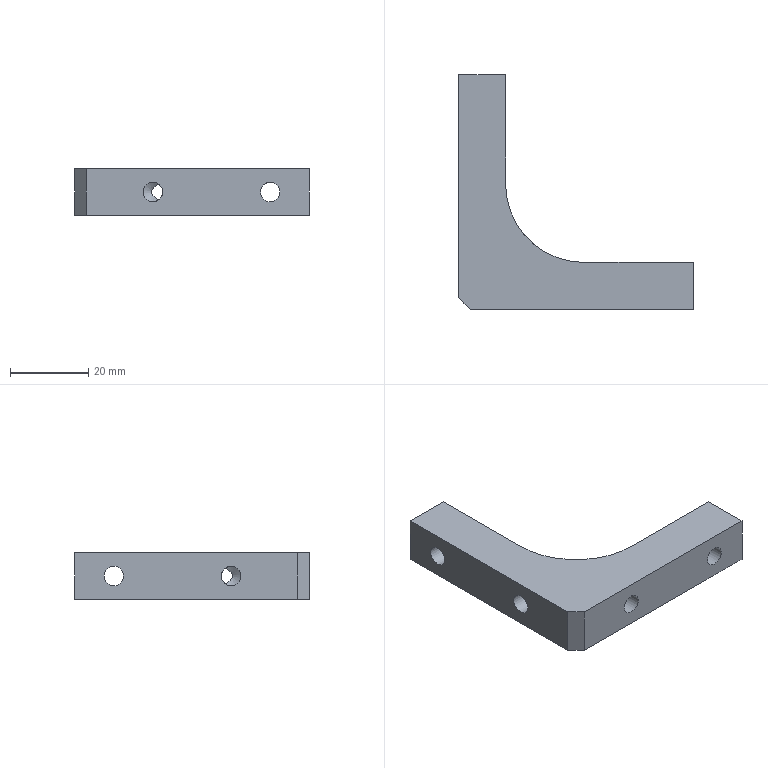Part | NX | 1 solid | 16 faces | box 60 x 60 x 12 mm | volume 15454 mm3 | plane 9 | cylinder 5 | cone 2 | commonest cylinder face diameters 5 x4 40 x1
STEP:
#1=CARTESIAN_POINT('',(12.,60.,-6.));
#2=VERTEX_POINT('',#1);
#3=CARTESIAN_POINT('',(0.,60.,-6.));
#4=VERTEX_POINT('',#3);
#5=CARTESIAN_POINT('',(12.,60.,-6.));
#6=DIRECTION('',(-1.,0.,0.));
#7=VECTOR('',#6,1000.);
#8=LINE('',#5,#7);
#9=EDGE_CURVE('',#2,#4,#8,.T.);
#10=ORIENTED_EDGE('',*,*,#9,.T.);
#11=CARTESIAN_POINT('',(0.,60.,6.));
#12=VERTEX_POINT('',#11);
#13=CARTESIAN_POINT('',(0.,60.,6.));
#14=DIRECTION('',(0.,0.,-1.));
#15=VECTOR('',#14,1000.);
#16=LINE('',#13,#15);
#17=EDGE_CURVE('',#12,#4,#16,.T.);
#18=ORIENTED_EDGE('',*,*,#17,.F.);
#19=CARTESIAN_POINT('',(12.,60.,6.));
#20=VERTEX_POINT('',#19);
#21=CARTESIAN_POINT('',(12.,60.,6.));
#22=DIRECTION('',(-1.,0.,0.));
#23=VECTOR('',#22,1000.);
#24=LINE('',#21,#23);
#25=EDGE_CURVE('',#20,#12,#24,.T.);
#26=ORIENTED_EDGE('',*,*,#25,.F.);
#27=CARTESIAN_POINT('',(12.,60.,6.));
#28=DIRECTION('',(0.,0.,-1.));
#29=VECTOR('',#28,1000.);
#30=LINE('',#27,#29);
#31=EDGE_CURVE('',#20,#2,#30,.T.);
#32=ORIENTED_EDGE('',*,*,#31,.T.);
#33=EDGE_LOOP('',(#10,#18,#26,#32));
#34=FACE_BOUND('',#33,.T.);
#35=CARTESIAN_POINT('',(12.,60.,6.));
#36=DIRECTION('',(0.,-1.,0.));
#37=DIRECTION('',(1.,0.,0.));
#38=AXIS2_PLACEMENT_3D('',#35,#36,#37);
#39=PLANE('',#38);
#40=ADVANCED_FACE('',(#34),#39,.F.);
#41=CARTESIAN_POINT('',(0.,20.,2.5));
#42=VERTEX_POINT('',#41);
#43=CARTESIAN_POINT('',(0.,20.,0.));
#44=DIRECTION('',(-1.,0.,0.));
#45=DIRECTION('',(0.,0.,1.));
#46=AXIS2_PLACEMENT_3D('',#43,#44,#45);
#47=CIRCLE('',#46,2.5);
#48=EDGE_CURVE('',#42,#42,#47,.T.);
#49=ORIENTED_EDGE('',*,*,#48,.F.);
#50=EDGE_LOOP('',(#49));
#51=FACE_BOUND('',#50,.T.);
#52=CARTESIAN_POINT('',(0.,50.,2.5));
#53=VERTEX_POINT('',#52);
#54=CARTESIAN_POINT('',(0.,50.,0.));
#55=DIRECTION('',(-1.,0.,0.));
#56=DIRECTION('',(0.,0.,1.));
#57=AXIS2_PLACEMENT_3D('',#54,#55,#56);
#58=CIRCLE('',#57,2.5);
#59=EDGE_CURVE('',#53,#53,#58,.T.);
#60=ORIENTED_EDGE('',*,*,#59,.F.);
#61=EDGE_LOOP('',(#60));
#62=FACE_BOUND('',#61,.T.);
#63=CARTESIAN_POINT('',(0.,3.,-6.));
#64=VERTEX_POINT('',#63);
#65=CARTESIAN_POINT('',(0.,60.,-6.));
#66=DIRECTION('',(0.,-1.,0.));
#67=VECTOR('',#66,1000.);
#68=LINE('',#65,#67);
#69=EDGE_CURVE('',#4,#64,#68,.T.);
#70=ORIENTED_EDGE('',*,*,#69,.T.);
#71=CARTESIAN_POINT('',(0.,3.,6.));
#72=VERTEX_POINT('',#71);
#73=CARTESIAN_POINT('',(0.,3.,6.));
#74=DIRECTION('',(0.,0.,1.));
#75=VECTOR('',#74,1000.);
#76=LINE('',#73,#75);
#77=EDGE_CURVE('',#64,#72,#76,.T.);
#78=ORIENTED_EDGE('',*,*,#77,.T.);
#79=CARTESIAN_POINT('',(0.,60.,6.));
#80=DIRECTION('',(0.,-1.,0.));
#81=VECTOR('',#80,1000.);
#82=LINE('',#79,#81);
#83=EDGE_CURVE('',#12,#72,#82,.T.);
#84=ORIENTED_EDGE('',*,*,#83,.F.);
#85=ORIENTED_EDGE('',*,*,#17,.T.);
#86=EDGE_LOOP('',(#70,#78,#84,#85));
#87=FACE_BOUND('',#86,.T.);
#88=CARTESIAN_POINT('',(0.,60.,6.));
#89=DIRECTION('',(1.,0.,0.));
#90=DIRECTION('',(0.,1.,0.));
#91=AXIS2_PLACEMENT_3D('',#88,#89,#90);
#92=PLANE('',#91);
#93=ADVANCED_FACE('',(#51,#62,#87),#92,.F.);
#94=CARTESIAN_POINT('',(20.,0.,-2.5));
#95=VERTEX_POINT('',#94);
#96=CARTESIAN_POINT('',(20.,0.,0.));
#97=DIRECTION('',(0.,-1.,0.));
#98=DIRECTION('',(0.,0.,-1.));
#99=AXIS2_PLACEMENT_3D('',#96,#97,#98);
#100=CIRCLE('',#99,2.5);
#101=EDGE_CURVE('',#95,#95,#100,.T.);
#102=ORIENTED_EDGE('',*,*,#101,.F.);
#103=EDGE_LOOP('',(#102));
#104=FACE_BOUND('',#103,.T.);
#105=CARTESIAN_POINT('',(50.,0.,-2.5));
#106=VERTEX_POINT('',#105);
#107=CARTESIAN_POINT('',(50.,0.,0.));
#108=DIRECTION('',(0.,-1.,0.));
#109=DIRECTION('',(0.,0.,-1.));
#110=AXIS2_PLACEMENT_3D('',#107,#108,#109);
#111=CIRCLE('',#110,2.5);
#112=EDGE_CURVE('',#106,#106,#111,.T.);
#113=ORIENTED_EDGE('',*,*,#112,.F.);
#114=EDGE_LOOP('',(#113));
#115=FACE_BOUND('',#114,.T.);
#116=CARTESIAN_POINT('',(3.,0.,6.));
#117=VERTEX_POINT('',#116);
#118=CARTESIAN_POINT('',(60.,0.,6.));
#119=VERTEX_POINT('',#118);
#120=CARTESIAN_POINT('',(0.,0.,6.));
#121=DIRECTION('',(1.,0.,0.));
#122=VECTOR('',#121,1000.);
#123=LINE('',#120,#122);
#124=EDGE_CURVE('',#117,#119,#123,.T.);
#125=ORIENTED_EDGE('',*,*,#124,.F.);
#126=CARTESIAN_POINT('',(3.,0.,-6.));
#127=VERTEX_POINT('',#126);
#128=CARTESIAN_POINT('',(3.,0.,6.));
#129=DIRECTION('',(0.,0.,-1.));
#130=VECTOR('',#129,1000.);
#131=LINE('',#128,#130);
#132=EDGE_CURVE('',#117,#127,#131,.T.);
#133=ORIENTED_EDGE('',*,*,#132,.T.);
#134=CARTESIAN_POINT('',(60.,0.,-6.));
#135=VERTEX_POINT('',#134);
#136=CARTESIAN_POINT('',(0.,0.,-6.));
#137=DIRECTION('',(1.,0.,0.));
#138=VECTOR('',#137,1000.);
#139=LINE('',#136,#138);
#140=EDGE_CURVE('',#127,#135,#139,.T.);
#141=ORIENTED_EDGE('',*,*,#140,.T.);
#142=CARTESIAN_POINT('',(60.,0.,6.));
#143=DIRECTION('',(0.,0.,-1.));
#144=VECTOR('',#143,1000.);
#145=LINE('',#142,#144);
#146=EDGE_CURVE('',#119,#135,#145,.T.);
#147=ORIENTED_EDGE('',*,*,#146,.F.);
#148=EDGE_LOOP('',(#125,#133,#141,#147));
#149=FACE_BOUND('',#148,.T.);
#150=CARTESIAN_POINT('',(0.,0.,6.));
#151=DIRECTION('',(0.,1.,0.));
#152=DIRECTION('',(-1.,0.,0.));
#153=AXIS2_PLACEMENT_3D('',#150,#151,#152);
#154=PLANE('',#153);
#155=ADVANCED_FACE('',(#104,#115,#149),#154,.F.);
#156=CARTESIAN_POINT('',(60.,12.,-6.));
#157=VERTEX_POINT('',#156);
#158=CARTESIAN_POINT('',(60.,0.,-6.));
#159=DIRECTION('',(0.,1.,0.));
#160=VECTOR('',#159,1000.);
#161=LINE('',#158,#160);
#162=EDGE_CURVE('',#135,#157,#161,.T.);
#163=ORIENTED_EDGE('',*,*,#162,.T.);
#164=CARTESIAN_POINT('',(60.,12.,6.));
#165=VERTEX_POINT('',#164);
#166=CARTESIAN_POINT('',(60.,12.,6.));
#167=DIRECTION('',(0.,0.,-1.));
#168=VECTOR('',#167,1000.);
#169=LINE('',#166,#168);
#170=EDGE_CURVE('',#165,#157,#169,.T.);
#171=ORIENTED_EDGE('',*,*,#170,.F.);
#172=CARTESIAN_POINT('',(60.,0.,6.));
#173=DIRECTION('',(0.,1.,0.));
#174=VECTOR('',#173,1000.);
#175=LINE('',#172,#174);
#176=EDGE_CURVE('',#119,#165,#175,.T.);
#177=ORIENTED_EDGE('',*,*,#176,.F.);
#178=ORIENTED_EDGE('',*,*,#146,.T.);
#179=EDGE_LOOP('',(#163,#171,#177,#178));
#180=FACE_BOUND('',#179,.T.);
#181=CARTESIAN_POINT('',(60.,0.,6.));
#182=DIRECTION('',(-1.,0.,0.));
#183=DIRECTION('',(0.,-1.,0.));
#184=AXIS2_PLACEMENT_3D('',#181,#182,#183);
#185=PLANE('',#184);
#186=ADVANCED_FACE('',(#180),#185,.F.);
#187=CARTESIAN_POINT('',(52.5,12.,0.));
#188=VERTEX_POINT('',#187);
#189=CARTESIAN_POINT('',(50.,12.,0.));
#190=DIRECTION('',(0.,-1.,0.));
#191=DIRECTION('',(1.,0.,0.));
#192=AXIS2_PLACEMENT_3D('',#189,#190,#191);
#193=CIRCLE('',#192,2.5);
#194=EDGE_CURVE('',#188,#188,#193,.T.);
#195=ORIENTED_EDGE('',*,*,#194,.T.);
#196=EDGE_LOOP('',(#195));
#197=FACE_BOUND('',#196,.T.);
#198=CARTESIAN_POINT('',(32.,12.,-6.));
#199=VERTEX_POINT('',#198);
#200=CARTESIAN_POINT('',(60.,12.,-6.));
#201=DIRECTION('',(-1.,0.,0.));
#202=VECTOR('',#201,1000.);
#203=LINE('',#200,#202);
#204=EDGE_CURVE('',#157,#199,#203,.T.);
#205=ORIENTED_EDGE('',*,*,#204,.T.);
#206=CARTESIAN_POINT('',(32.,12.,6.));
#207=VERTEX_POINT('',#206);
#208=CARTESIAN_POINT('',(32.,12.,6.));
#209=DIRECTION('',(0.,0.,-1.));
#210=VECTOR('',#209,1000.);
#211=LINE('',#208,#210);
#212=EDGE_CURVE('',#199,#207,#211,.F.);
#213=ORIENTED_EDGE('',*,*,#212,.T.);
#214=CARTESIAN_POINT('',(60.,12.,6.));
#215=DIRECTION('',(-1.,0.,0.));
#216=VECTOR('',#215,1000.);
#217=LINE('',#214,#216);
#218=EDGE_CURVE('',#165,#207,#217,.T.);
#219=ORIENTED_EDGE('',*,*,#218,.F.);
#220=ORIENTED_EDGE('',*,*,#170,.T.);
#221=EDGE_LOOP('',(#205,#213,#219,#220));
#222=FACE_BOUND('',#221,.T.);
#223=CARTESIAN_POINT('',(60.,12.,6.));
#224=DIRECTION('',(0.,-1.,0.));
#225=DIRECTION('',(1.,0.,0.));
#226=AXIS2_PLACEMENT_3D('',#223,#224,#225);
#227=PLANE('',#226);
#228=ADVANCED_FACE('',(#197,#222),#227,.F.);
#229=CARTESIAN_POINT('',(12.,50.,2.5));
#230=VERTEX_POINT('',#229);
#231=CARTESIAN_POINT('',(12.,50.,0.));
#232=DIRECTION('',(-1.,0.,0.));
#233=DIRECTION('',(0.,0.,1.));
#234=AXIS2_PLACEMENT_3D('',#231,#232,#233);
#235=CIRCLE('',#234,2.5);
#236=EDGE_CURVE('',#230,#230,#235,.T.);
#237=ORIENTED_EDGE('',*,*,#236,.T.);
#238=EDGE_LOOP('',(#237));
#239=FACE_BOUND('',#238,.T.);
#240=CARTESIAN_POINT('',(12.,32.,6.));
#241=VERTEX_POINT('',#240);
#242=CARTESIAN_POINT('',(12.,12.,6.));
#243=DIRECTION('',(0.,1.,0.));
#244=VECTOR('',#243,1000.);
#245=LINE('',#242,#244);
#246=EDGE_CURVE('',#241,#20,#245,.T.);
#247=ORIENTED_EDGE('',*,*,#246,.F.);
#248=CARTESIAN_POINT('',(12.,32.,-6.));
#249=VERTEX_POINT('',#248);
#250=CARTESIAN_POINT('',(12.,32.,-6.));
#251=DIRECTION('',(0.,0.,-1.));
#252=VECTOR('',#251,1000.);
#253=LINE('',#250,#252);
#254=EDGE_CURVE('',#241,#249,#253,.T.);
#255=ORIENTED_EDGE('',*,*,#254,.T.);
#256=CARTESIAN_POINT('',(12.,12.,-6.));
#257=DIRECTION('',(0.,1.,0.));
#258=VECTOR('',#257,1000.);
#259=LINE('',#256,#258);
#260=EDGE_CURVE('',#249,#2,#259,.T.);
#261=ORIENTED_EDGE('',*,*,#260,.T.);
#262=ORIENTED_EDGE('',*,*,#31,.F.);
#263=EDGE_LOOP('',(#247,#255,#261,#262));
#264=FACE_BOUND('',#263,.T.);
#265=CARTESIAN_POINT('',(12.,12.,6.));
#266=DIRECTION('',(-1.,0.,0.));
#267=DIRECTION('',(0.,0.,1.));
#268=AXIS2_PLACEMENT_3D('',#265,#266,#267);
#269=PLANE('',#268);
#270=ADVANCED_FACE('',(#239,#264),#269,.F.);
#271=ORIENTED_EDGE('',*,*,#83,.T.);
#272=CARTESIAN_POINT('',(1.5,1.5,6.));
#273=DIRECTION('',(-0.7071,0.7071,0.));
#274=VECTOR('',#273,1000.);
#275=LINE('',#272,#274);
#276=EDGE_CURVE('',#72,#117,#275,.F.);
#277=ORIENTED_EDGE('',*,*,#276,.T.);
#278=ORIENTED_EDGE('',*,*,#124,.T.);
#279=ORIENTED_EDGE('',*,*,#176,.T.);
#280=ORIENTED_EDGE('',*,*,#218,.T.);
#281=CARTESIAN_POINT('',(32.,32.,6.));
#282=DIRECTION('',(0.,0.,1.));
#283=DIRECTION('',(1.,0.,0.));
#284=AXIS2_PLACEMENT_3D('',#281,#282,#283);
#285=CIRCLE('',#284,20.);
#286=EDGE_CURVE('',#207,#241,#285,.F.);
#287=ORIENTED_EDGE('',*,*,#286,.T.);
#288=ORIENTED_EDGE('',*,*,#246,.T.);
#289=ORIENTED_EDGE('',*,*,#25,.T.);
#290=EDGE_LOOP('',(#271,#277,#278,#279,#280,#287,#288,#289));
#291=FACE_BOUND('',#290,.T.);
#292=CARTESIAN_POINT('',(0.,0.,6.));
#293=DIRECTION('',(0.,0.,1.));
#294=DIRECTION('',(1.,0.,0.));
#295=AXIS2_PLACEMENT_3D('',#292,#293,#294);
#296=PLANE('',#295);
#297=ADVANCED_FACE('',(#291),#296,.T.);
#298=ORIENTED_EDGE('',*,*,#140,.F.);
#299=CARTESIAN_POINT('',(3.,0.,-6.));
#300=DIRECTION('',(0.7071,-0.7071,0.));
#301=VECTOR('',#300,1000.);
#302=LINE('',#299,#301);
#303=EDGE_CURVE('',#127,#64,#302,.F.);
#304=ORIENTED_EDGE('',*,*,#303,.T.);
#305=ORIENTED_EDGE('',*,*,#69,.F.);
#306=ORIENTED_EDGE('',*,*,#9,.F.);
#307=ORIENTED_EDGE('',*,*,#260,.F.);
#308=CARTESIAN_POINT('',(32.,32.,-6.));
#309=DIRECTION('',(0.,0.,1.));
#310=DIRECTION('',(1.,0.,0.));
#311=AXIS2_PLACEMENT_3D('',#308,#309,#310);
#312=CIRCLE('',#311,20.);
#313=EDGE_CURVE('',#249,#199,#312,.T.);
#314=ORIENTED_EDGE('',*,*,#313,.T.);
#315=ORIENTED_EDGE('',*,*,#204,.F.);
#316=ORIENTED_EDGE('',*,*,#162,.F.);
#317=EDGE_LOOP('',(#298,#304,#305,#306,#307,#314,#315,#316));
#318=FACE_BOUND('',#317,.T.);
#319=CARTESIAN_POINT('',(0.,0.,-6.));
#320=DIRECTION('',(0.,0.,1.));
#321=DIRECTION('',(1.,0.,0.));
#322=AXIS2_PLACEMENT_3D('',#319,#320,#321);
#323=PLANE('',#322);
#324=ADVANCED_FACE('',(#318),#323,.F.);
#325=CARTESIAN_POINT('',(21.464,15.,2.026));
#326=VERTEX_POINT('',#325);
#327=CARTESIAN_POINT('',(21.464,15.,-2.026));
#328=VERTEX_POINT('',#327);
#329=CARTESIAN_POINT('',(21.464,15.,2.026));
#330=CARTESIAN_POINT('',(21.064,15.248,1.806));
#331=CARTESIAN_POINT('',(20.513,15.619,1.402));
#332=CARTESIAN_POINT('',(19.878,16.089,0.737));
#333=CARTESIAN_POINT('',(19.511,16.378,0.003696));
#334=CARTESIAN_POINT('',(19.876,16.09,-0.7352));
#335=CARTESIAN_POINT('',(20.504,15.625,-1.393));
#336=CARTESIAN_POINT('',(21.064,15.248,-1.806));
#337=CARTESIAN_POINT('',(21.464,15.,-2.026));
#338=B_SPLINE_CURVE_WITH_KNOTS('',3,(#329,#330,#331,#332,#333,#334,#335,#336,#337),.UNSPECIFIED.,.F.,.F.,(4,1,1,1,1,1,4),(0.0003121,0.00186,0.002633,0.003407,0.004181,0.004954,0.006502),.UNSPECIFIED.);
#339=EDGE_CURVE('',#326,#328,#338,.T.);
#340=ORIENTED_EDGE('',*,*,#339,.T.);
#341=CARTESIAN_POINT('',(21.464,15.,-2.026));
#342=CARTESIAN_POINT('',(22.063,14.629,-1.594));
#343=CARTESIAN_POINT('',(22.937,14.172,-0.004795));
#344=CARTESIAN_POINT('',(22.063,14.629,1.593));
#345=CARTESIAN_POINT('',(21.464,15.,2.026));
#346=B_SPLINE_CURVE_WITH_KNOTS('',3,(#341,#342,#343,#344,#345),.UNSPECIFIED.,.F.,.F.,(4,1,4),(0.,0.002449,0.004897),.UNSPECIFIED.);
#347=EDGE_CURVE('',#328,#326,#346,.T.);
#348=ORIENTED_EDGE('',*,*,#347,.T.);
#349=EDGE_LOOP('',(#340,#348));
#350=FACE_BOUND('',#349,.T.);
#351=CARTESIAN_POINT('',(15.,21.464,-2.026));
#352=VERTEX_POINT('',#351);
#353=CARTESIAN_POINT('',(15.,21.464,2.026));
#354=VERTEX_POINT('',#353);
#355=CARTESIAN_POINT('',(15.,21.464,-2.026));
#356=CARTESIAN_POINT('',(15.248,21.064,-1.806));
#357=CARTESIAN_POINT('',(15.619,20.513,-1.402));
#358=CARTESIAN_POINT('',(16.089,19.878,-0.737));
#359=CARTESIAN_POINT('',(16.378,19.511,-0.003696));
#360=CARTESIAN_POINT('',(16.09,19.876,0.7352));
#361=CARTESIAN_POINT('',(15.625,20.504,1.393));
#362=CARTESIAN_POINT('',(15.248,21.064,1.806));
#363=CARTESIAN_POINT('',(15.,21.464,2.026));
#364=B_SPLINE_CURVE_WITH_KNOTS('',3,(#355,#356,#357,#358,#359,#360,#361,#362,#363),.UNSPECIFIED.,.F.,.F.,(4,1,1,1,1,1,4),(0.0003121,0.00186,0.002633,0.003407,0.004181,0.004954,0.006502),.UNSPECIFIED.);
#365=EDGE_CURVE('',#352,#354,#364,.T.);
#366=ORIENTED_EDGE('',*,*,#365,.T.);
#367=CARTESIAN_POINT('',(15.,21.464,2.026));
#368=CARTESIAN_POINT('',(14.629,22.063,1.594));
#369=CARTESIAN_POINT('',(14.172,22.937,0.004795));
#370=CARTESIAN_POINT('',(14.629,22.063,-1.593));
#371=CARTESIAN_POINT('',(15.,21.464,-2.026));
#372=B_SPLINE_CURVE_WITH_KNOTS('',3,(#367,#368,#369,#370,#371),.UNSPECIFIED.,.F.,.F.,(4,1,4),(0.,0.002449,0.004897),.UNSPECIFIED.);
#373=EDGE_CURVE('',#354,#352,#372,.T.);
#374=ORIENTED_EDGE('',*,*,#373,.T.);
#375=EDGE_LOOP('',(#366,#374));
#376=FACE_BOUND('',#375,.T.);
#377=ORIENTED_EDGE('',*,*,#286,.F.);
#378=ORIENTED_EDGE('',*,*,#212,.F.);
#379=ORIENTED_EDGE('',*,*,#313,.F.);
#380=ORIENTED_EDGE('',*,*,#254,.F.);
#381=EDGE_LOOP('',(#377,#378,#379,#380));
#382=FACE_BOUND('',#381,.T.);
#383=CARTESIAN_POINT('',(32.,32.,6.));
#384=DIRECTION('',(0.,0.,1.));
#385=DIRECTION('',(1.,0.,0.));
#386=AXIS2_PLACEMENT_3D('',#383,#384,#385);
#387=CYLINDRICAL_SURFACE('',#386,20.);
#388=ADVANCED_FACE('',(#350,#376,#382),#387,.F.);
#389=ORIENTED_EDGE('',*,*,#59,.T.);
#390=EDGE_LOOP('',(#389));
#391=FACE_BOUND('',#390,.T.);
#392=ORIENTED_EDGE('',*,*,#236,.F.);
#393=EDGE_LOOP('',(#392));
#394=FACE_BOUND('',#393,.T.);
#395=CARTESIAN_POINT('',(0.,50.,0.));
#396=DIRECTION('',(-1.,0.,0.));
#397=DIRECTION('',(0.,0.,1.));
#398=AXIS2_PLACEMENT_3D('',#395,#396,#397);
#399=CYLINDRICAL_SURFACE('',#398,2.5);
#400=ADVANCED_FACE('',(#391,#394),#399,.F.);
#401=ORIENTED_EDGE('',*,*,#48,.T.);
#402=EDGE_LOOP('',(#401));
#403=FACE_BOUND('',#402,.T.);
#404=CARTESIAN_POINT('',(15.,20.,0.));
#405=DIRECTION('',(-1.,0.,0.));
#406=DIRECTION('',(0.,0.,1.));
#407=AXIS2_PLACEMENT_3D('',#404,#405,#406);
#408=CIRCLE('',#407,2.5);
#409=EDGE_CURVE('',#352,#354,#408,.T.);
#410=ORIENTED_EDGE('',*,*,#409,.F.);
#411=ORIENTED_EDGE('',*,*,#373,.F.);
#412=EDGE_LOOP('',(#410,#411));
#413=FACE_BOUND('',#412,.T.);
#414=CARTESIAN_POINT('',(0.,20.,0.));
#415=DIRECTION('',(-1.,0.,0.));
#416=DIRECTION('',(0.,0.,1.));
#417=AXIS2_PLACEMENT_3D('',#414,#415,#416);
#418=CYLINDRICAL_SURFACE('',#417,2.5);
#419=ADVANCED_FACE('',(#403,#413),#418,.F.);
#420=ORIENTED_EDGE('',*,*,#409,.T.);
#421=ORIENTED_EDGE('',*,*,#365,.F.);
#422=EDGE_LOOP('',(#420,#421));
#423=FACE_BOUND('',#422,.T.);
#424=CARTESIAN_POINT('',(15.,20.,0.));
#425=DIRECTION('',(-1.,0.,0.));
#426=DIRECTION('',(0.,0.,1.));
#427=AXIS2_PLACEMENT_3D('',#424,#425,#426);
#428=CONICAL_SURFACE('',#427,2.5,1.03);
#429=ADVANCED_FACE('',(#423),#428,.F.);
#430=ORIENTED_EDGE('',*,*,#112,.T.);
#431=EDGE_LOOP('',(#430));
#432=FACE_BOUND('',#431,.T.);
#433=ORIENTED_EDGE('',*,*,#194,.F.);
#434=EDGE_LOOP('',(#433));
#435=FACE_BOUND('',#434,.T.);
#436=CARTESIAN_POINT('',(50.,0.,0.));
#437=DIRECTION('',(0.,-1.,0.));
#438=DIRECTION('',(0.,0.,-1.));
#439=AXIS2_PLACEMENT_3D('',#436,#437,#438);
#440=CYLINDRICAL_SURFACE('',#439,2.5);
#441=ADVANCED_FACE('',(#432,#435),#440,.F.);
#442=ORIENTED_EDGE('',*,*,#101,.T.);
#443=EDGE_LOOP('',(#442));
#444=FACE_BOUND('',#443,.T.);
#445=CARTESIAN_POINT('',(20.,15.,0.));
#446=DIRECTION('',(0.,-1.,0.));
#447=DIRECTION('',(0.,0.,-1.));
#448=AXIS2_PLACEMENT_3D('',#445,#446,#447);
#449=CIRCLE('',#448,2.5);
#450=EDGE_CURVE('',#326,#328,#449,.T.);
#451=ORIENTED_EDGE('',*,*,#450,.F.);
#452=ORIENTED_EDGE('',*,*,#347,.F.);
#453=EDGE_LOOP('',(#451,#452));
#454=FACE_BOUND('',#453,.T.);
#455=CARTESIAN_POINT('',(20.,0.,0.));
#456=DIRECTION('',(0.,-1.,0.));
#457=DIRECTION('',(0.,0.,-1.));
#458=AXIS2_PLACEMENT_3D('',#455,#456,#457);
#459=CYLINDRICAL_SURFACE('',#458,2.5);
#460=ADVANCED_FACE('',(#444,#454),#459,.F.);
#461=ORIENTED_EDGE('',*,*,#450,.T.);
#462=ORIENTED_EDGE('',*,*,#339,.F.);
#463=EDGE_LOOP('',(#461,#462));
#464=FACE_BOUND('',#463,.T.);
#465=CARTESIAN_POINT('',(20.,15.,0.));
#466=DIRECTION('',(0.,-1.,0.));
#467=DIRECTION('',(0.,0.,-1.));
#468=AXIS2_PLACEMENT_3D('',#465,#466,#467);
#469=CONICAL_SURFACE('',#468,2.5,1.03);
#470=ADVANCED_FACE('',(#464),#469,.F.);
#471=ORIENTED_EDGE('',*,*,#276,.F.);
#472=ORIENTED_EDGE('',*,*,#77,.F.);
#473=ORIENTED_EDGE('',*,*,#303,.F.);
#474=ORIENTED_EDGE('',*,*,#132,.F.);
#475=EDGE_LOOP('',(#471,#472,#473,#474));
#476=FACE_BOUND('',#475,.T.);
#477=CARTESIAN_POINT('',(3.,0.,6.));
#478=DIRECTION('',(0.7071,0.7071,0.));
#479=DIRECTION('',(0.,0.,-1.));
#480=AXIS2_PLACEMENT_3D('',#477,#478,#479);
#481=PLANE('',#480);
#482=ADVANCED_FACE('',(#476),#481,.F.);
#483=CLOSED_SHELL('',(#40,#93,#155,#186,#228,#270,#297,#324,#388,#400,#419,#429,#441,#460,#470,#482));
#484=MANIFOLD_SOLID_BREP('',#483);
#485=(LENGTH_UNIT()NAMED_UNIT(*)SI_UNIT(.MILLI.,.METRE.));
#486=UNCERTAINTY_MEASURE_WITH_UNIT(LENGTH_MEASURE(0.0508),#485,'','');
#487=(NAMED_UNIT(*)PLANE_ANGLE_UNIT()SI_UNIT($,.RADIAN.));
#488=(NAMED_UNIT(*)SI_UNIT($,.STERADIAN.)SOLID_ANGLE_UNIT());
#489=(GEOMETRIC_REPRESENTATION_CONTEXT(3)GLOBAL_UNCERTAINTY_ASSIGNED_CONTEXT((#486))GLOBAL_UNIT_ASSIGNED_CONTEXT((#485,#487,#488))REPRESENTATION_CONTEXT('',''));
#490=ADVANCED_BREP_SHAPE_REPRESENTATION('',(#484),#489);